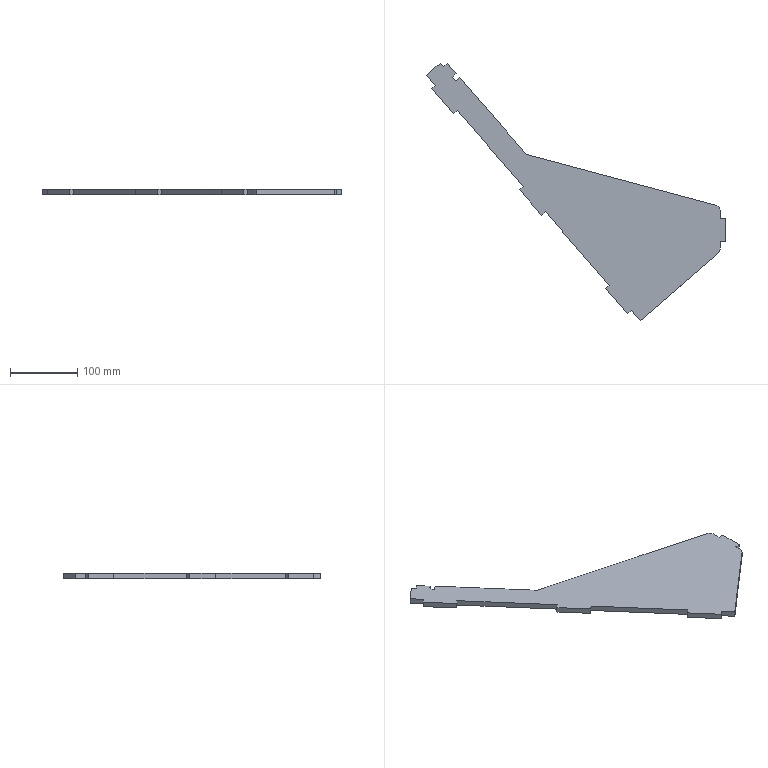Part | SolidWorks | features FlatPattern 1, SMBaseFlange 1, SheetMetal 1 | 1 solid | 33 faces | box 445.432 x 383.748 x 8 mm | volume 369427 mm3 | plane 30 | cylinder 3 | commonest cylinder face diameters 20 x2 4 x1
STEP:
#1=CARTESIAN_POINT('',(-13.039,-561.326,0.));
#2=VERTEX_POINT('',#1);
#3=CARTESIAN_POINT('',(-9.6,-553.779,0.));
#4=VERTEX_POINT('',#3);
#5=CARTESIAN_POINT('',(-19.6,-553.779,0.));
#6=DIRECTION('',(0.,0.,1.));
#7=DIRECTION('',(1.,0.,0.));
#8=AXIS2_PLACEMENT_3D('',#5,#6,#7);
#9=CIRCLE('',#8,10.);
#10=EDGE_CURVE('',#2,#4,#9,.T.);
#11=ORIENTED_EDGE('',*,*,#10,.F.);
#12=CARTESIAN_POINT('',(-13.039,-561.326,-8.));
#13=VERTEX_POINT('',#12);
#14=CARTESIAN_POINT('',(-13.039,-561.326,-8.));
#15=DIRECTION('',(0.,0.,1.));
#16=VECTOR('',#15,1000.);
#17=LINE('',#14,#16);
#18=EDGE_CURVE('',#13,#2,#17,.T.);
#19=ORIENTED_EDGE('',*,*,#18,.F.);
#20=CARTESIAN_POINT('',(-9.6,-553.779,-8.));
#21=VERTEX_POINT('',#20);
#22=CARTESIAN_POINT('',(-19.6,-553.779,-8.));
#23=DIRECTION('',(0.,0.,1.));
#24=DIRECTION('',(1.,0.,0.));
#25=AXIS2_PLACEMENT_3D('',#22,#23,#24);
#26=CIRCLE('',#25,10.);
#27=EDGE_CURVE('',#13,#21,#26,.T.);
#28=ORIENTED_EDGE('',*,*,#27,.T.);
#29=CARTESIAN_POINT('',(-9.6,-553.779,-8.));
#30=DIRECTION('',(0.,0.,1.));
#31=VECTOR('',#30,1000.);
#32=LINE('',#29,#31);
#33=EDGE_CURVE('',#21,#4,#32,.T.);
#34=ORIENTED_EDGE('',*,*,#33,.T.);
#35=EDGE_LOOP('',(#11,#19,#28,#34));
#36=FACE_OUTER_BOUND('',#35,.T.);
#37=CARTESIAN_POINT('',(-19.6,-553.779,-8.));
#38=DIRECTION('',(0.,0.,1.));
#39=DIRECTION('',(1.,0.,0.));
#40=AXIS2_PLACEMENT_3D('',#37,#38,#39);
#41=CYLINDRICAL_SURFACE('',#40,10.);
#42=ADVANCED_FACE('',(#36),#41,.T.);
#43=CARTESIAN_POINT('',(-129.344,-662.428,0.));
#44=VERTEX_POINT('',#43);
#45=CARTESIAN_POINT('',(-13.039,-561.326,0.));
#46=DIRECTION('',(0.7547,0.6561,0.));
#47=VECTOR('',#46,1000.);
#48=LINE('',#45,#47);
#49=EDGE_CURVE('',#44,#2,#48,.T.);
#50=ORIENTED_EDGE('',*,*,#49,.F.);
#51=CARTESIAN_POINT('',(-129.344,-662.428,-8.));
#52=VERTEX_POINT('',#51);
#53=CARTESIAN_POINT('',(-129.344,-662.428,-8.));
#54=DIRECTION('',(0.,0.,1.));
#55=VECTOR('',#54,1000.);
#56=LINE('',#53,#55);
#57=EDGE_CURVE('',#52,#44,#56,.T.);
#58=ORIENTED_EDGE('',*,*,#57,.F.);
#59=CARTESIAN_POINT('',(-13.039,-561.326,-8.));
#60=DIRECTION('',(0.7547,0.6561,0.));
#61=VECTOR('',#60,1000.);
#62=LINE('',#59,#61);
#63=EDGE_CURVE('',#52,#13,#62,.T.);
#64=ORIENTED_EDGE('',*,*,#63,.T.);
#65=ORIENTED_EDGE('',*,*,#18,.T.);
#66=EDGE_LOOP('',(#50,#58,#64,#65));
#67=FACE_OUTER_BOUND('',#66,.T.);
#68=CARTESIAN_POINT('',(-13.039,-561.326,-8.));
#69=DIRECTION('',(0.6561,-0.7547,0.));
#70=DIRECTION('',(0.7547,0.6561,0.));
#71=AXIS2_PLACEMENT_3D('',#68,#69,#70);
#72=PLANE('',#71);
#73=ADVANCED_FACE('',(#67),#72,.T.);
#74=CARTESIAN_POINT('',(-142.465,-647.333,0.));
#75=VERTEX_POINT('',#74);
#76=CARTESIAN_POINT('',(-142.465,-647.333,0.));
#77=DIRECTION('',(0.6561,-0.7547,0.));
#78=VECTOR('',#77,1000.);
#79=LINE('',#76,#78);
#80=EDGE_CURVE('',#75,#44,#79,.T.);
#81=ORIENTED_EDGE('',*,*,#80,.F.);
#82=CARTESIAN_POINT('',(-142.465,-647.333,-8.));
#83=VERTEX_POINT('',#82);
#84=CARTESIAN_POINT('',(-142.465,-647.333,-8.));
#85=DIRECTION('',(0.,0.,1.));
#86=VECTOR('',#85,1000.);
#87=LINE('',#84,#86);
#88=EDGE_CURVE('',#83,#75,#87,.T.);
#89=ORIENTED_EDGE('',*,*,#88,.F.);
#90=CARTESIAN_POINT('',(-142.465,-647.333,-8.));
#91=DIRECTION('',(0.6561,-0.7547,0.));
#92=VECTOR('',#91,1000.);
#93=LINE('',#90,#92);
#94=EDGE_CURVE('',#83,#52,#93,.T.);
#95=ORIENTED_EDGE('',*,*,#94,.T.);
#96=ORIENTED_EDGE('',*,*,#57,.T.);
#97=EDGE_LOOP('',(#81,#89,#95,#96));
#98=FACE_OUTER_BOUND('',#97,.T.);
#99=CARTESIAN_POINT('',(-142.465,-647.333,-8.));
#100=DIRECTION('',(-0.7547,-0.6561,0.));
#101=DIRECTION('',(0.6561,-0.7547,0.));
#102=AXIS2_PLACEMENT_3D('',#99,#100,#101);
#103=PLANE('',#102);
#104=ADVANCED_FACE('',(#98),#103,.T.);
#105=CARTESIAN_POINT('',(-148.125,-652.254,0.));
#106=VERTEX_POINT('',#105);
#107=CARTESIAN_POINT('',(-142.465,-647.333,0.));
#108=DIRECTION('',(0.7547,0.6561,0.));
#109=VECTOR('',#108,1000.);
#110=LINE('',#107,#109);
#111=EDGE_CURVE('',#106,#75,#110,.T.);
#112=ORIENTED_EDGE('',*,*,#111,.F.);
#113=CARTESIAN_POINT('',(-148.125,-652.254,-8.));
#114=VERTEX_POINT('',#113);
#115=CARTESIAN_POINT('',(-148.125,-652.254,-8.));
#116=DIRECTION('',(0.,0.,1.));
#117=VECTOR('',#116,1000.);
#118=LINE('',#115,#117);
#119=EDGE_CURVE('',#114,#106,#118,.T.);
#120=ORIENTED_EDGE('',*,*,#119,.F.);
#121=CARTESIAN_POINT('',(-142.465,-647.333,-8.));
#122=DIRECTION('',(0.7547,0.6561,0.));
#123=VECTOR('',#122,1000.);
#124=LINE('',#121,#123);
#125=EDGE_CURVE('',#114,#83,#124,.T.);
#126=ORIENTED_EDGE('',*,*,#125,.T.);
#127=ORIENTED_EDGE('',*,*,#88,.T.);
#128=EDGE_LOOP('',(#112,#120,#126,#127));
#129=FACE_OUTER_BOUND('',#128,.T.);
#130=CARTESIAN_POINT('',(-142.465,-647.333,-8.));
#131=DIRECTION('',(0.6561,-0.7547,0.));
#132=DIRECTION('',(0.7547,0.6561,0.));
#133=AXIS2_PLACEMENT_3D('',#130,#131,#132);
#134=PLANE('',#133);
#135=ADVANCED_FACE('',(#129),#134,.T.);
#136=CARTESIAN_POINT('',(-180.928,-614.518,0.));
#137=VERTEX_POINT('',#136);
#138=CARTESIAN_POINT('',(-148.125,-652.254,0.));
#139=DIRECTION('',(0.6561,-0.7547,0.));
#140=VECTOR('',#139,1000.);
#141=LINE('',#138,#140);
#142=EDGE_CURVE('',#137,#106,#141,.T.);
#143=ORIENTED_EDGE('',*,*,#142,.F.);
#144=CARTESIAN_POINT('',(-180.928,-614.518,-8.));
#145=VERTEX_POINT('',#144);
#146=CARTESIAN_POINT('',(-180.928,-614.518,-8.));
#147=DIRECTION('',(0.,0.,1.));
#148=VECTOR('',#147,1000.);
#149=LINE('',#146,#148);
#150=EDGE_CURVE('',#145,#137,#149,.T.);
#151=ORIENTED_EDGE('',*,*,#150,.F.);
#152=CARTESIAN_POINT('',(-148.125,-652.254,-8.));
#153=DIRECTION('',(0.6561,-0.7547,0.));
#154=VECTOR('',#153,1000.);
#155=LINE('',#152,#154);
#156=EDGE_CURVE('',#145,#114,#155,.T.);
#157=ORIENTED_EDGE('',*,*,#156,.T.);
#158=ORIENTED_EDGE('',*,*,#119,.T.);
#159=EDGE_LOOP('',(#143,#151,#157,#158));
#160=FACE_OUTER_BOUND('',#159,.T.);
#161=CARTESIAN_POINT('',(-148.125,-652.254,-8.));
#162=DIRECTION('',(-0.7547,-0.6561,0.));
#163=DIRECTION('',(0.6561,-0.7547,0.));
#164=AXIS2_PLACEMENT_3D('',#161,#162,#163);
#165=PLANE('',#164);
#166=ADVANCED_FACE('',(#160),#165,.T.);
#167=CARTESIAN_POINT('',(-175.268,-609.598,0.));
#168=VERTEX_POINT('',#167);
#169=CARTESIAN_POINT('',(-180.928,-614.518,0.));
#170=DIRECTION('',(-0.7547,-0.6561,0.));
#171=VECTOR('',#170,1000.);
#172=LINE('',#169,#171);
#173=EDGE_CURVE('',#168,#137,#172,.T.);
#174=ORIENTED_EDGE('',*,*,#173,.F.);
#175=CARTESIAN_POINT('',(-175.268,-609.598,-8.));
#176=VERTEX_POINT('',#175);
#177=CARTESIAN_POINT('',(-175.268,-609.598,-8.));
#178=DIRECTION('',(0.,0.,1.));
#179=VECTOR('',#178,1000.);
#180=LINE('',#177,#179);
#181=EDGE_CURVE('',#176,#168,#180,.T.);
#182=ORIENTED_EDGE('',*,*,#181,.F.);
#183=CARTESIAN_POINT('',(-180.928,-614.518,-8.));
#184=DIRECTION('',(-0.7547,-0.6561,0.));
#185=VECTOR('',#184,1000.);
#186=LINE('',#183,#185);
#187=EDGE_CURVE('',#176,#145,#186,.T.);
#188=ORIENTED_EDGE('',*,*,#187,.T.);
#189=ORIENTED_EDGE('',*,*,#150,.T.);
#190=EDGE_LOOP('',(#174,#182,#188,#189));
#191=FACE_OUTER_BOUND('',#190,.T.);
#192=CARTESIAN_POINT('',(-180.928,-614.518,-8.));
#193=DIRECTION('',(-0.6561,0.7547,0.));
#194=DIRECTION('',(-0.7547,-0.6561,0.));
#195=AXIS2_PLACEMENT_3D('',#192,#193,#194);
#196=PLANE('',#195);
#197=ADVANCED_FACE('',(#191),#196,.T.);
#198=CARTESIAN_POINT('',(-270.396,-500.165,0.));
#199=VERTEX_POINT('',#198);
#200=CARTESIAN_POINT('',(-270.396,-500.165,0.));
#201=DIRECTION('',(0.6561,-0.7547,0.));
#202=VECTOR('',#201,1000.);
#203=LINE('',#200,#202);
#204=EDGE_CURVE('',#199,#168,#203,.T.);
#205=ORIENTED_EDGE('',*,*,#204,.F.);
#206=CARTESIAN_POINT('',(-270.396,-500.165,-8.));
#207=VERTEX_POINT('',#206);
#208=CARTESIAN_POINT('',(-270.396,-500.165,-8.));
#209=DIRECTION('',(0.,0.,1.));
#210=VECTOR('',#209,1000.);
#211=LINE('',#208,#210);
#212=EDGE_CURVE('',#207,#199,#211,.T.);
#213=ORIENTED_EDGE('',*,*,#212,.F.);
#214=CARTESIAN_POINT('',(-270.396,-500.165,-8.));
#215=DIRECTION('',(0.6561,-0.7547,0.));
#216=VECTOR('',#215,1000.);
#217=LINE('',#214,#216);
#218=EDGE_CURVE('',#207,#176,#217,.T.);
#219=ORIENTED_EDGE('',*,*,#218,.T.);
#220=ORIENTED_EDGE('',*,*,#181,.T.);
#221=EDGE_LOOP('',(#205,#213,#219,#220));
#222=FACE_OUTER_BOUND('',#221,.T.);
#223=CARTESIAN_POINT('',(-270.396,-500.165,-8.));
#224=DIRECTION('',(-0.7547,-0.6561,0.));
#225=DIRECTION('',(0.6561,-0.7547,0.));
#226=AXIS2_PLACEMENT_3D('',#223,#224,#225);
#227=PLANE('',#226);
#228=ADVANCED_FACE('',(#222),#227,.T.);
#229=CARTESIAN_POINT('',(-276.057,-505.085,0.));
#230=VERTEX_POINT('',#229);
#231=CARTESIAN_POINT('',(-276.057,-505.085,0.));
#232=DIRECTION('',(0.7547,0.6561,0.));
#233=VECTOR('',#232,1000.);
#234=LINE('',#231,#233);
#235=EDGE_CURVE('',#230,#199,#234,.T.);
#236=ORIENTED_EDGE('',*,*,#235,.F.);
#237=CARTESIAN_POINT('',(-276.057,-505.085,-8.));
#238=VERTEX_POINT('',#237);
#239=CARTESIAN_POINT('',(-276.057,-505.085,-8.));
#240=DIRECTION('',(0.,0.,1.));
#241=VECTOR('',#240,1000.);
#242=LINE('',#239,#241);
#243=EDGE_CURVE('',#238,#230,#242,.T.);
#244=ORIENTED_EDGE('',*,*,#243,.F.);
#245=CARTESIAN_POINT('',(-276.057,-505.085,-8.));
#246=DIRECTION('',(0.7547,0.6561,0.));
#247=VECTOR('',#246,1000.);
#248=LINE('',#245,#247);
#249=EDGE_CURVE('',#238,#207,#248,.T.);
#250=ORIENTED_EDGE('',*,*,#249,.T.);
#251=ORIENTED_EDGE('',*,*,#212,.T.);
#252=EDGE_LOOP('',(#236,#244,#250,#251));
#253=FACE_OUTER_BOUND('',#252,.T.);
#254=CARTESIAN_POINT('',(-276.057,-505.085,-8.));
#255=DIRECTION('',(0.6561,-0.7547,0.));
#256=DIRECTION('',(0.7547,0.6561,0.));
#257=AXIS2_PLACEMENT_3D('',#254,#255,#256);
#258=PLANE('',#257);
#259=ADVANCED_FACE('',(#253),#258,.T.);
#260=CARTESIAN_POINT('',(-308.86,-467.35,0.));
#261=VERTEX_POINT('',#260);
#262=CARTESIAN_POINT('',(-308.86,-467.35,0.));
#263=DIRECTION('',(0.6561,-0.7547,0.));
#264=VECTOR('',#263,1000.);
#265=LINE('',#262,#264);
#266=EDGE_CURVE('',#261,#230,#265,.T.);
#267=ORIENTED_EDGE('',*,*,#266,.F.);
#268=CARTESIAN_POINT('',(-308.86,-467.35,-8.));
#269=VERTEX_POINT('',#268);
#270=CARTESIAN_POINT('',(-308.86,-467.35,-8.));
#271=DIRECTION('',(0.,0.,1.));
#272=VECTOR('',#271,1000.);
#273=LINE('',#270,#272);
#274=EDGE_CURVE('',#269,#261,#273,.T.);
#275=ORIENTED_EDGE('',*,*,#274,.F.);
#276=CARTESIAN_POINT('',(-308.86,-467.35,-8.));
#277=DIRECTION('',(0.6561,-0.7547,0.));
#278=VECTOR('',#277,1000.);
#279=LINE('',#276,#278);
#280=EDGE_CURVE('',#269,#238,#279,.T.);
#281=ORIENTED_EDGE('',*,*,#280,.T.);
#282=ORIENTED_EDGE('',*,*,#243,.T.);
#283=EDGE_LOOP('',(#267,#275,#281,#282));
#284=FACE_OUTER_BOUND('',#283,.T.);
#285=CARTESIAN_POINT('',(-308.86,-467.35,-8.));
#286=DIRECTION('',(-0.7547,-0.6561,0.));
#287=DIRECTION('',(0.6561,-0.7547,0.));
#288=AXIS2_PLACEMENT_3D('',#285,#286,#287);
#289=PLANE('',#288);
#290=ADVANCED_FACE('',(#284),#289,.T.);
#291=CARTESIAN_POINT('',(-303.199,-462.429,0.));
#292=VERTEX_POINT('',#291);
#293=CARTESIAN_POINT('',(-303.199,-462.429,0.));
#294=DIRECTION('',(-0.7547,-0.6561,0.));
#295=VECTOR('',#294,1000.);
#296=LINE('',#293,#295);
#297=EDGE_CURVE('',#292,#261,#296,.T.);
#298=ORIENTED_EDGE('',*,*,#297,.F.);
#299=CARTESIAN_POINT('',(-303.199,-462.429,-8.));
#300=VERTEX_POINT('',#299);
#301=CARTESIAN_POINT('',(-303.199,-462.429,-8.));
#302=DIRECTION('',(0.,0.,1.));
#303=VECTOR('',#302,1000.);
#304=LINE('',#301,#303);
#305=EDGE_CURVE('',#300,#292,#304,.T.);
#306=ORIENTED_EDGE('',*,*,#305,.F.);
#307=CARTESIAN_POINT('',(-303.199,-462.429,-8.));
#308=DIRECTION('',(-0.7547,-0.6561,0.));
#309=VECTOR('',#308,1000.);
#310=LINE('',#307,#309);
#311=EDGE_CURVE('',#300,#269,#310,.T.);
#312=ORIENTED_EDGE('',*,*,#311,.T.);
#313=ORIENTED_EDGE('',*,*,#274,.T.);
#314=EDGE_LOOP('',(#298,#306,#312,#313));
#315=FACE_OUTER_BOUND('',#314,.T.);
#316=CARTESIAN_POINT('',(-303.199,-462.429,-8.));
#317=DIRECTION('',(-0.6561,0.7547,0.));
#318=DIRECTION('',(-0.7547,-0.6561,0.));
#319=AXIS2_PLACEMENT_3D('',#316,#317,#318);
#320=PLANE('',#319);
#321=ADVANCED_FACE('',(#315),#320,.T.);
#322=CARTESIAN_POINT('',(-401.608,-349.223,0.));
#323=VERTEX_POINT('',#322);
#324=CARTESIAN_POINT('',(-401.608,-349.223,0.));
#325=DIRECTION('',(0.6561,-0.7547,0.));
#326=VECTOR('',#325,1000.);
#327=LINE('',#324,#326);
#328=EDGE_CURVE('',#323,#292,#327,.T.);
#329=ORIENTED_EDGE('',*,*,#328,.F.);
#330=CARTESIAN_POINT('',(-401.608,-349.223,-8.));
#331=VERTEX_POINT('',#330);
#332=CARTESIAN_POINT('',(-401.608,-349.223,-8.));
#333=DIRECTION('',(0.,0.,1.));
#334=VECTOR('',#333,1000.);
#335=LINE('',#332,#334);
#336=EDGE_CURVE('',#331,#323,#335,.T.);
#337=ORIENTED_EDGE('',*,*,#336,.F.);
#338=CARTESIAN_POINT('',(-401.608,-349.223,-8.));
#339=DIRECTION('',(0.6561,-0.7547,0.));
#340=VECTOR('',#339,1000.);
#341=LINE('',#338,#340);
#342=EDGE_CURVE('',#331,#300,#341,.T.);
#343=ORIENTED_EDGE('',*,*,#342,.T.);
#344=ORIENTED_EDGE('',*,*,#305,.T.);
#345=EDGE_LOOP('',(#329,#337,#343,#344));
#346=FACE_OUTER_BOUND('',#345,.T.);
#347=CARTESIAN_POINT('',(-401.608,-349.223,-8.));
#348=DIRECTION('',(-0.7547,-0.6561,0.));
#349=DIRECTION('',(0.6561,-0.7547,0.));
#350=AXIS2_PLACEMENT_3D('',#347,#348,#349);
#351=PLANE('',#350);
#352=ADVANCED_FACE('',(#346),#351,.T.);
#353=CARTESIAN_POINT('',(-407.269,-354.143,0.));
#354=VERTEX_POINT('',#353);
#355=CARTESIAN_POINT('',(-407.269,-354.143,0.));
#356=DIRECTION('',(0.7547,0.6561,0.));
#357=VECTOR('',#356,1000.);
#358=LINE('',#355,#357);
#359=EDGE_CURVE('',#354,#323,#358,.T.);
#360=ORIENTED_EDGE('',*,*,#359,.F.);
#361=CARTESIAN_POINT('',(-407.269,-354.143,-8.));
#362=VERTEX_POINT('',#361);
#363=CARTESIAN_POINT('',(-407.269,-354.143,-8.));
#364=DIRECTION('',(0.,0.,1.));
#365=VECTOR('',#364,1000.);
#366=LINE('',#363,#365);
#367=EDGE_CURVE('',#362,#354,#366,.T.);
#368=ORIENTED_EDGE('',*,*,#367,.F.);
#369=CARTESIAN_POINT('',(-407.269,-354.143,-8.));
#370=DIRECTION('',(0.7547,0.6561,0.));
#371=VECTOR('',#370,1000.);
#372=LINE('',#369,#371);
#373=EDGE_CURVE('',#362,#331,#372,.T.);
#374=ORIENTED_EDGE('',*,*,#373,.T.);
#375=ORIENTED_EDGE('',*,*,#336,.T.);
#376=EDGE_LOOP('',(#360,#368,#374,#375));
#377=FACE_OUTER_BOUND('',#376,.T.);
#378=CARTESIAN_POINT('',(-407.269,-354.143,-8.));
#379=DIRECTION('',(0.6561,-0.7547,0.));
#380=DIRECTION('',(0.7547,0.6561,0.));
#381=AXIS2_PLACEMENT_3D('',#378,#379,#380);
#382=PLANE('',#381);
#383=ADVANCED_FACE('',(#377),#382,.T.);
#384=CARTESIAN_POINT('',(-440.071,-316.408,0.));
#385=VERTEX_POINT('',#384);
#386=CARTESIAN_POINT('',(-440.071,-316.408,0.));
#387=DIRECTION('',(0.6561,-0.7547,0.));
#388=VECTOR('',#387,1000.);
#389=LINE('',#386,#388);
#390=EDGE_CURVE('',#385,#354,#389,.T.);
#391=ORIENTED_EDGE('',*,*,#390,.F.);
#392=CARTESIAN_POINT('',(-440.071,-316.408,-8.));
#393=VERTEX_POINT('',#392);
#394=CARTESIAN_POINT('',(-440.071,-316.408,-8.));
#395=DIRECTION('',(0.,0.,1.));
#396=VECTOR('',#395,1000.);
#397=LINE('',#394,#396);
#398=EDGE_CURVE('',#393,#385,#397,.T.);
#399=ORIENTED_EDGE('',*,*,#398,.F.);
#400=CARTESIAN_POINT('',(-440.071,-316.408,-8.));
#401=DIRECTION('',(0.6561,-0.7547,0.));
#402=VECTOR('',#401,1000.);
#403=LINE('',#400,#402);
#404=EDGE_CURVE('',#393,#362,#403,.T.);
#405=ORIENTED_EDGE('',*,*,#404,.T.);
#406=ORIENTED_EDGE('',*,*,#367,.T.);
#407=EDGE_LOOP('',(#391,#399,#405,#406));
#408=FACE_OUTER_BOUND('',#407,.T.);
#409=CARTESIAN_POINT('',(-440.071,-316.408,-8.));
#410=DIRECTION('',(-0.7547,-0.6561,0.));
#411=DIRECTION('',(0.6561,-0.7547,0.));
#412=AXIS2_PLACEMENT_3D('',#409,#410,#411);
#413=PLANE('',#412);
#414=ADVANCED_FACE('',(#408),#413,.T.);
#415=CARTESIAN_POINT('',(-434.411,-311.488,0.));
#416=VERTEX_POINT('',#415);
#417=CARTESIAN_POINT('',(-434.411,-311.488,0.));
#418=DIRECTION('',(-0.7547,-0.6561,0.));
#419=VECTOR('',#418,1000.);
#420=LINE('',#417,#419);
#421=EDGE_CURVE('',#416,#385,#420,.T.);
#422=ORIENTED_EDGE('',*,*,#421,.F.);
#423=CARTESIAN_POINT('',(-434.411,-311.488,-8.));
#424=VERTEX_POINT('',#423);
#425=CARTESIAN_POINT('',(-434.411,-311.488,-8.));
#426=DIRECTION('',(0.,0.,1.));
#427=VECTOR('',#426,1000.);
#428=LINE('',#425,#427);
#429=EDGE_CURVE('',#424,#416,#428,.T.);
#430=ORIENTED_EDGE('',*,*,#429,.F.);
#431=CARTESIAN_POINT('',(-434.411,-311.488,-8.));
#432=DIRECTION('',(-0.7547,-0.6561,0.));
#433=VECTOR('',#432,1000.);
#434=LINE('',#431,#433);
#435=EDGE_CURVE('',#424,#393,#434,.T.);
#436=ORIENTED_EDGE('',*,*,#435,.T.);
#437=ORIENTED_EDGE('',*,*,#398,.T.);
#438=EDGE_LOOP('',(#422,#430,#436,#437));
#439=FACE_OUTER_BOUND('',#438,.T.);
#440=CARTESIAN_POINT('',(-434.411,-311.488,-8.));
#441=DIRECTION('',(-0.6561,0.7547,0.));
#442=DIRECTION('',(-0.7547,-0.6561,0.));
#443=AXIS2_PLACEMENT_3D('',#440,#441,#442);
#444=PLANE('',#443);
#445=ADVANCED_FACE('',(#439),#444,.T.);
#446=CARTESIAN_POINT('',(-447.532,-296.393,0.));
#447=VERTEX_POINT('',#446);
#448=CARTESIAN_POINT('',(-447.532,-296.393,0.));
#449=DIRECTION('',(0.6561,-0.7547,0.));
#450=VECTOR('',#449,1000.);
#451=LINE('',#448,#450);
#452=EDGE_CURVE('',#447,#416,#451,.T.);
#453=ORIENTED_EDGE('',*,*,#452,.F.);
#454=CARTESIAN_POINT('',(-447.532,-296.393,-8.));
#455=VERTEX_POINT('',#454);
#456=CARTESIAN_POINT('',(-447.532,-296.393,-8.));
#457=DIRECTION('',(0.,0.,1.));
#458=VECTOR('',#457,1000.);
#459=LINE('',#456,#458);
#460=EDGE_CURVE('',#455,#447,#459,.T.);
#461=ORIENTED_EDGE('',*,*,#460,.F.);
#462=CARTESIAN_POINT('',(-447.532,-296.393,-8.));
#463=DIRECTION('',(0.6561,-0.7547,0.));
#464=VECTOR('',#463,1000.);
#465=LINE('',#462,#464);
#466=EDGE_CURVE('',#455,#424,#465,.T.);
#467=ORIENTED_EDGE('',*,*,#466,.T.);
#468=ORIENTED_EDGE('',*,*,#429,.T.);
#469=EDGE_LOOP('',(#453,#461,#467,#468));
#470=FACE_OUTER_BOUND('',#469,.T.);
#471=CARTESIAN_POINT('',(-447.532,-296.393,-8.));
#472=DIRECTION('',(-0.7547,-0.6561,0.));
#473=DIRECTION('',(0.6561,-0.7547,0.));
#474=AXIS2_PLACEMENT_3D('',#471,#472,#473);
#475=PLANE('',#474);
#476=ADVANCED_FACE('',(#470),#475,.T.);
#477=CARTESIAN_POINT('',(-427.155,-278.68,0.));
#478=VERTEX_POINT('',#477);
#479=CARTESIAN_POINT('',(-427.155,-278.68,0.));
#480=DIRECTION('',(-0.7547,-0.6561,0.));
#481=VECTOR('',#480,1000.);
#482=LINE('',#479,#481);
#483=EDGE_CURVE('',#478,#447,#482,.T.);
#484=ORIENTED_EDGE('',*,*,#483,.F.);
#485=CARTESIAN_POINT('',(-427.155,-278.68,-8.));
#486=VERTEX_POINT('',#485);
#487=CARTESIAN_POINT('',(-427.155,-278.68,-8.));
#488=DIRECTION('',(0.,0.,1.));
#489=VECTOR('',#488,1000.);
#490=LINE('',#487,#489);
#491=EDGE_CURVE('',#486,#478,#490,.T.);
#492=ORIENTED_EDGE('',*,*,#491,.F.);
#493=CARTESIAN_POINT('',(-427.155,-278.68,-8.));
#494=DIRECTION('',(-0.7547,-0.6561,0.));
#495=VECTOR('',#494,1000.);
#496=LINE('',#493,#495);
#497=EDGE_CURVE('',#486,#455,#496,.T.);
#498=ORIENTED_EDGE('',*,*,#497,.T.);
#499=ORIENTED_EDGE('',*,*,#460,.T.);
#500=EDGE_LOOP('',(#484,#492,#498,#499));
#501=FACE_OUTER_BOUND('',#500,.T.);
#502=CARTESIAN_POINT('',(-427.155,-278.68,-8.));
#503=DIRECTION('',(-0.6561,0.7547,0.));
#504=DIRECTION('',(-0.7547,-0.6561,0.));
#505=AXIS2_PLACEMENT_3D('',#502,#503,#504);
#506=PLANE('',#505);
#507=ADVANCED_FACE('',(#501),#506,.T.);
#508=CARTESIAN_POINT('',(-422.235,-284.34,0.));
#509=VERTEX_POINT('',#508);
#510=CARTESIAN_POINT('',(-427.155,-278.68,0.));
#511=DIRECTION('',(-0.6561,0.7547,0.));
#512=VECTOR('',#511,1000.);
#513=LINE('',#510,#512);
#514=EDGE_CURVE('',#509,#478,#513,.T.);
#515=ORIENTED_EDGE('',*,*,#514,.F.);
#516=CARTESIAN_POINT('',(-422.235,-284.34,-8.));
#517=VERTEX_POINT('',#516);
#518=CARTESIAN_POINT('',(-422.235,-284.34,-8.));
#519=DIRECTION('',(0.,0.,1.));
#520=VECTOR('',#519,1000.);
#521=LINE('',#518,#520);
#522=EDGE_CURVE('',#517,#509,#521,.T.);
#523=ORIENTED_EDGE('',*,*,#522,.F.);
#524=CARTESIAN_POINT('',(-427.155,-278.68,-8.));
#525=DIRECTION('',(-0.6561,0.7547,0.));
#526=VECTOR('',#525,1000.);
#527=LINE('',#524,#526);
#528=EDGE_CURVE('',#517,#486,#527,.T.);
#529=ORIENTED_EDGE('',*,*,#528,.T.);
#530=ORIENTED_EDGE('',*,*,#491,.T.);
#531=EDGE_LOOP('',(#515,#523,#529,#530));
#532=FACE_OUTER_BOUND('',#531,.T.);
#533=CARTESIAN_POINT('',(-427.155,-278.68,-8.));
#534=DIRECTION('',(0.7547,0.6561,0.));
#535=DIRECTION('',(-0.6561,0.7547,0.));
#536=AXIS2_PLACEMENT_3D('',#533,#534,#535);
#537=PLANE('',#536);
#538=ADVANCED_FACE('',(#532),#537,.T.);
#539=CARTESIAN_POINT('',(-416.574,-279.42,0.));
#540=VERTEX_POINT('',#539);
#541=CARTESIAN_POINT('',(-422.235,-284.34,0.));
#542=DIRECTION('',(-0.7547,-0.6561,0.));
#543=VECTOR('',#542,1000.);
#544=LINE('',#541,#543);
#545=EDGE_CURVE('',#540,#509,#544,.T.);
#546=ORIENTED_EDGE('',*,*,#545,.F.);
#547=CARTESIAN_POINT('',(-416.574,-279.42,-8.));
#548=VERTEX_POINT('',#547);
#549=CARTESIAN_POINT('',(-416.574,-279.42,-8.));
#550=DIRECTION('',(0.,0.,1.));
#551=VECTOR('',#550,1000.);
#552=LINE('',#549,#551);
#553=EDGE_CURVE('',#548,#540,#552,.T.);
#554=ORIENTED_EDGE('',*,*,#553,.F.);
#555=CARTESIAN_POINT('',(-422.235,-284.34,-8.));
#556=DIRECTION('',(-0.7547,-0.6561,0.));
#557=VECTOR('',#556,1000.);
#558=LINE('',#555,#557);
#559=EDGE_CURVE('',#548,#517,#558,.T.);
#560=ORIENTED_EDGE('',*,*,#559,.T.);
#561=ORIENTED_EDGE('',*,*,#522,.T.);
#562=EDGE_LOOP('',(#546,#554,#560,#561));
#563=FACE_OUTER_BOUND('',#562,.T.);
#564=CARTESIAN_POINT('',(-422.235,-284.34,-8.));
#565=DIRECTION('',(-0.6561,0.7547,0.));
#566=DIRECTION('',(-0.7547,-0.6561,0.));
#567=AXIS2_PLACEMENT_3D('',#564,#565,#566);
#568=PLANE('',#567);
#569=ADVANCED_FACE('',(#563),#568,.T.);
#570=CARTESIAN_POINT('',(-403.453,-294.514,0.));
#571=VERTEX_POINT('',#570);
#572=CARTESIAN_POINT('',(-416.574,-279.42,0.));
#573=DIRECTION('',(-0.6561,0.7547,0.));
#574=VECTOR('',#573,1000.);
#575=LINE('',#572,#574);
#576=EDGE_CURVE('',#571,#540,#575,.T.);
#577=ORIENTED_EDGE('',*,*,#576,.F.);
#578=CARTESIAN_POINT('',(-403.453,-294.514,-8.));
#579=VERTEX_POINT('',#578);
#580=CARTESIAN_POINT('',(-403.453,-294.514,-8.));
#581=DIRECTION('',(0.,0.,1.));
#582=VECTOR('',#581,1000.);
#583=LINE('',#580,#582);
#584=EDGE_CURVE('',#579,#571,#583,.T.);
#585=ORIENTED_EDGE('',*,*,#584,.F.);
#586=CARTESIAN_POINT('',(-416.574,-279.42,-8.));
#587=DIRECTION('',(-0.6561,0.7547,0.));
#588=VECTOR('',#587,1000.);
#589=LINE('',#586,#588);
#590=EDGE_CURVE('',#579,#548,#589,.T.);
#591=ORIENTED_EDGE('',*,*,#590,.T.);
#592=ORIENTED_EDGE('',*,*,#553,.T.);
#593=EDGE_LOOP('',(#577,#585,#591,#592));
#594=FACE_OUTER_BOUND('',#593,.T.);
#595=CARTESIAN_POINT('',(-416.574,-279.42,-8.));
#596=DIRECTION('',(0.7547,0.6561,0.));
#597=DIRECTION('',(-0.6561,0.7547,0.));
#598=AXIS2_PLACEMENT_3D('',#595,#596,#597);
#599=PLANE('',#598);
#600=ADVANCED_FACE('',(#594),#599,.T.);
#601=CARTESIAN_POINT('',(-409.114,-299.434,0.));
#602=VERTEX_POINT('',#601);
#603=CARTESIAN_POINT('',(-403.453,-294.514,0.));
#604=DIRECTION('',(0.7547,0.6561,0.));
#605=VECTOR('',#604,1000.);
#606=LINE('',#603,#605);
#607=EDGE_CURVE('',#602,#571,#606,.T.);
#608=ORIENTED_EDGE('',*,*,#607,.F.);
#609=CARTESIAN_POINT('',(-409.114,-299.434,-8.));
#610=VERTEX_POINT('',#609);
#611=CARTESIAN_POINT('',(-409.114,-299.434,-8.));
#612=DIRECTION('',(0.,0.,1.));
#613=VECTOR('',#612,1000.);
#614=LINE('',#611,#613);
#615=EDGE_CURVE('',#610,#602,#614,.T.);
#616=ORIENTED_EDGE('',*,*,#615,.F.);
#617=CARTESIAN_POINT('',(-403.453,-294.514,-8.));
#618=DIRECTION('',(0.7547,0.6561,0.));
#619=VECTOR('',#618,1000.);
#620=LINE('',#617,#619);
#621=EDGE_CURVE('',#610,#579,#620,.T.);
#622=ORIENTED_EDGE('',*,*,#621,.T.);
#623=ORIENTED_EDGE('',*,*,#584,.T.);
#624=EDGE_LOOP('',(#608,#616,#622,#623));
#625=FACE_OUTER_BOUND('',#624,.T.);
#626=CARTESIAN_POINT('',(-403.453,-294.514,-8.));
#627=DIRECTION('',(0.6561,-0.7547,0.));
#628=DIRECTION('',(0.7547,0.6561,0.));
#629=AXIS2_PLACEMENT_3D('',#626,#627,#628);
#630=PLANE('',#629);
#631=ADVANCED_FACE('',(#625),#630,.T.);
#632=CARTESIAN_POINT('',(-404.193,-305.095,0.));
#633=VERTEX_POINT('',#632);
#634=CARTESIAN_POINT('',(-409.114,-299.434,0.));
#635=DIRECTION('',(-0.6561,0.7547,0.));
#636=VECTOR('',#635,1000.);
#637=LINE('',#634,#636);
#638=EDGE_CURVE('',#633,#602,#637,.T.);
#639=ORIENTED_EDGE('',*,*,#638,.F.);
#640=CARTESIAN_POINT('',(-404.193,-305.095,-8.));
#641=VERTEX_POINT('',#640);
#642=CARTESIAN_POINT('',(-404.193,-305.095,-8.));
#643=DIRECTION('',(0.,0.,1.));
#644=VECTOR('',#643,1000.);
#645=LINE('',#642,#644);
#646=EDGE_CURVE('',#641,#633,#645,.T.);
#647=ORIENTED_EDGE('',*,*,#646,.F.);
#648=CARTESIAN_POINT('',(-409.114,-299.434,-8.));
#649=DIRECTION('',(-0.6561,0.7547,0.));
#650=VECTOR('',#649,1000.);
#651=LINE('',#648,#650);
#652=EDGE_CURVE('',#641,#610,#651,.T.);
#653=ORIENTED_EDGE('',*,*,#652,.T.);
#654=ORIENTED_EDGE('',*,*,#615,.T.);
#655=EDGE_LOOP('',(#639,#647,#653,#654));
#656=FACE_OUTER_BOUND('',#655,.T.);
#657=CARTESIAN_POINT('',(-409.114,-299.434,-8.));
#658=DIRECTION('',(0.7547,0.6561,0.));
#659=DIRECTION('',(-0.6561,0.7547,0.));
#660=AXIS2_PLACEMENT_3D('',#657,#658,#659);
#661=PLANE('',#660);
#662=ADVANCED_FACE('',(#656),#661,.T.);
#663=CARTESIAN_POINT('',(-398.155,-299.846,0.));
#664=VERTEX_POINT('',#663);
#665=CARTESIAN_POINT('',(-404.193,-305.095,0.));
#666=DIRECTION('',(-0.7547,-0.6561,0.));
#667=VECTOR('',#666,1000.);
#668=LINE('',#665,#667);
#669=EDGE_CURVE('',#664,#633,#668,.T.);
#670=ORIENTED_EDGE('',*,*,#669,.F.);
#671=CARTESIAN_POINT('',(-398.155,-299.846,-8.));
#672=VERTEX_POINT('',#671);
#673=CARTESIAN_POINT('',(-398.155,-299.846,-8.));
#674=DIRECTION('',(0.,0.,1.));
#675=VECTOR('',#674,1000.);
#676=LINE('',#673,#675);
#677=EDGE_CURVE('',#672,#664,#676,.T.);
#678=ORIENTED_EDGE('',*,*,#677,.F.);
#679=CARTESIAN_POINT('',(-404.193,-305.095,-8.));
#680=DIRECTION('',(-0.7547,-0.6561,0.));
#681=VECTOR('',#680,1000.);
#682=LINE('',#679,#681);
#683=EDGE_CURVE('',#672,#641,#682,.T.);
#684=ORIENTED_EDGE('',*,*,#683,.T.);
#685=ORIENTED_EDGE('',*,*,#646,.T.);
#686=EDGE_LOOP('',(#670,#678,#684,#685));
#687=FACE_OUTER_BOUND('',#686,.T.);
#688=CARTESIAN_POINT('',(-404.193,-305.095,-8.));
#689=DIRECTION('',(-0.6561,0.7547,0.));
#690=DIRECTION('',(-0.7547,-0.6561,0.));
#691=AXIS2_PLACEMENT_3D('',#688,#689,#690);
#692=PLANE('',#691);
#693=ADVANCED_FACE('',(#687),#692,.T.);
#694=CARTESIAN_POINT('',(-298.63,-414.337,0.));
#695=VERTEX_POINT('',#694);
#696=CARTESIAN_POINT('',(-398.155,-299.846,0.));
#697=DIRECTION('',(-0.6561,0.7547,0.));
#698=VECTOR('',#697,1000.);
#699=LINE('',#696,#698);
#700=EDGE_CURVE('',#695,#664,#699,.T.);
#701=ORIENTED_EDGE('',*,*,#700,.F.);
#702=CARTESIAN_POINT('',(-298.63,-414.337,-8.));
#703=VERTEX_POINT('',#702);
#704=CARTESIAN_POINT('',(-298.63,-414.337,-8.));
#705=DIRECTION('',(0.,0.,1.));
#706=VECTOR('',#705,1000.);
#707=LINE('',#704,#706);
#708=EDGE_CURVE('',#703,#695,#707,.T.);
#709=ORIENTED_EDGE('',*,*,#708,.F.);
#710=CARTESIAN_POINT('',(-398.155,-299.846,-8.));
#711=DIRECTION('',(-0.6561,0.7547,0.));
#712=VECTOR('',#711,1000.);
#713=LINE('',#710,#712);
#714=EDGE_CURVE('',#703,#672,#713,.T.);
#715=ORIENTED_EDGE('',*,*,#714,.T.);
#716=ORIENTED_EDGE('',*,*,#677,.T.);
#717=EDGE_LOOP('',(#701,#709,#715,#716));
#718=FACE_OUTER_BOUND('',#717,.T.);
#719=CARTESIAN_POINT('',(-398.155,-299.846,-8.));
#720=DIRECTION('',(0.7547,0.6561,0.));
#721=DIRECTION('',(-0.6561,0.7547,0.));
#722=AXIS2_PLACEMENT_3D('',#719,#720,#721);
#723=PLANE('',#722);
#724=ADVANCED_FACE('',(#718),#723,.T.);
#725=CARTESIAN_POINT('',(-297.639,-414.956,0.));
#726=VERTEX_POINT('',#725);
#727=CARTESIAN_POINT('',(-297.121,-413.024,0.));
#728=DIRECTION('',(0.,0.,-1.));
#729=DIRECTION('',(-1.,0.,0.));
#730=AXIS2_PLACEMENT_3D('',#727,#728,#729);
#731=CIRCLE('',#730,2.);
#732=EDGE_CURVE('',#726,#695,#731,.T.);
#733=ORIENTED_EDGE('',*,*,#732,.F.);
#734=CARTESIAN_POINT('',(-297.639,-414.956,-8.));
#735=VERTEX_POINT('',#734);
#736=CARTESIAN_POINT('',(-297.639,-414.956,-8.));
#737=DIRECTION('',(0.,0.,1.));
#738=VECTOR('',#737,1000.);
#739=LINE('',#736,#738);
#740=EDGE_CURVE('',#735,#726,#739,.T.);
#741=ORIENTED_EDGE('',*,*,#740,.F.);
#742=CARTESIAN_POINT('',(-297.121,-413.024,-8.));
#743=DIRECTION('',(0.,0.,-1.));
#744=DIRECTION('',(-1.,0.,0.));
#745=AXIS2_PLACEMENT_3D('',#742,#743,#744);
#746=CIRCLE('',#745,2.);
#747=EDGE_CURVE('',#735,#703,#746,.T.);
#748=ORIENTED_EDGE('',*,*,#747,.T.);
#749=ORIENTED_EDGE('',*,*,#708,.T.);
#750=EDGE_LOOP('',(#733,#741,#748,#749));
#751=FACE_OUTER_BOUND('',#750,.T.);
#752=CARTESIAN_POINT('',(-297.121,-413.024,-8.));
#753=DIRECTION('',(0.,0.,1.));
#754=DIRECTION('',(1.,0.,0.));
#755=AXIS2_PLACEMENT_3D('',#752,#753,#754);
#756=CYLINDRICAL_SURFACE('',#755,2.);
#757=ADVANCED_FACE('',(#751),#756,.F.);
#758=CARTESIAN_POINT('',(-17.012,-490.15,0.));
#759=VERTEX_POINT('',#758);
#760=CARTESIAN_POINT('',(-297.639,-414.956,0.));
#761=DIRECTION('',(-0.9659,0.2588,0.));
#762=VECTOR('',#761,1000.);
#763=LINE('',#760,#762);
#764=EDGE_CURVE('',#759,#726,#763,.T.);
#765=ORIENTED_EDGE('',*,*,#764,.F.);
#766=CARTESIAN_POINT('',(-17.012,-490.15,-8.));
#767=VERTEX_POINT('',#766);
#768=CARTESIAN_POINT('',(-17.012,-490.15,-8.));
#769=DIRECTION('',(0.,0.,1.));
#770=VECTOR('',#769,1000.);
#771=LINE('',#768,#770);
#772=EDGE_CURVE('',#767,#759,#771,.T.);
#773=ORIENTED_EDGE('',*,*,#772,.F.);
#774=CARTESIAN_POINT('',(-297.639,-414.956,-8.));
#775=DIRECTION('',(-0.9659,0.2588,0.));
#776=VECTOR('',#775,1000.);
#777=LINE('',#774,#776);
#778=EDGE_CURVE('',#767,#735,#777,.T.);
#779=ORIENTED_EDGE('',*,*,#778,.T.);
#780=ORIENTED_EDGE('',*,*,#740,.T.);
#781=EDGE_LOOP('',(#765,#773,#779,#780));
#782=FACE_OUTER_BOUND('',#781,.T.);
#783=CARTESIAN_POINT('',(-297.639,-414.956,-8.));
#784=DIRECTION('',(0.2588,0.9659,0.));
#785=DIRECTION('',(-0.9659,0.2588,0.));
#786=AXIS2_PLACEMENT_3D('',#783,#784,#785);
#787=PLANE('',#786);
#788=ADVANCED_FACE('',(#782),#787,.T.);
#789=CARTESIAN_POINT('',(-9.6,-499.809,0.));
#790=VERTEX_POINT('',#789);
#791=CARTESIAN_POINT('',(-19.6,-499.809,0.));
#792=DIRECTION('',(0.,0.,1.));
#793=DIRECTION('',(1.,0.,0.));
#794=AXIS2_PLACEMENT_3D('',#791,#792,#793);
#795=CIRCLE('',#794,10.);
#796=EDGE_CURVE('',#790,#759,#795,.T.);
#797=ORIENTED_EDGE('',*,*,#796,.F.);
#798=CARTESIAN_POINT('',(-9.6,-499.809,-8.));
#799=VERTEX_POINT('',#798);
#800=CARTESIAN_POINT('',(-9.6,-499.809,-8.));
#801=DIRECTION('',(0.,0.,1.));
#802=VECTOR('',#801,1000.);
#803=LINE('',#800,#802);
#804=EDGE_CURVE('',#799,#790,#803,.T.);
#805=ORIENTED_EDGE('',*,*,#804,.F.);
#806=CARTESIAN_POINT('',(-19.6,-499.809,-8.));
#807=DIRECTION('',(0.,0.,1.));
#808=DIRECTION('',(1.,0.,0.));
#809=AXIS2_PLACEMENT_3D('',#806,#807,#808);
#810=CIRCLE('',#809,10.);
#811=EDGE_CURVE('',#799,#767,#810,.T.);
#812=ORIENTED_EDGE('',*,*,#811,.T.);
#813=ORIENTED_EDGE('',*,*,#772,.T.);
#814=EDGE_LOOP('',(#797,#805,#812,#813));
#815=FACE_OUTER_BOUND('',#814,.T.);
#816=CARTESIAN_POINT('',(-19.6,-499.809,-8.));
#817=DIRECTION('',(0.,0.,1.));
#818=DIRECTION('',(1.,0.,0.));
#819=AXIS2_PLACEMENT_3D('',#816,#817,#818);
#820=CYLINDRICAL_SURFACE('',#819,10.);
#821=ADVANCED_FACE('',(#815),#820,.T.);
#822=CARTESIAN_POINT('',(-9.6,-509.809,0.));
#823=VERTEX_POINT('',#822);
#824=CARTESIAN_POINT('',(-9.6,-499.809,0.));
#825=DIRECTION('',(0.,1.,0.));
#826=VECTOR('',#825,1000.);
#827=LINE('',#824,#826);
#828=EDGE_CURVE('',#823,#790,#827,.T.);
#829=ORIENTED_EDGE('',*,*,#828,.F.);
#830=CARTESIAN_POINT('',(-9.6,-509.809,-8.));
#831=VERTEX_POINT('',#830);
#832=CARTESIAN_POINT('',(-9.6,-509.809,-8.));
#833=DIRECTION('',(0.,0.,1.));
#834=VECTOR('',#833,1000.);
#835=LINE('',#832,#834);
#836=EDGE_CURVE('',#831,#823,#835,.T.);
#837=ORIENTED_EDGE('',*,*,#836,.F.);
#838=CARTESIAN_POINT('',(-9.6,-499.809,-8.));
#839=DIRECTION('',(0.,1.,0.));
#840=VECTOR('',#839,1000.);
#841=LINE('',#838,#840);
#842=EDGE_CURVE('',#831,#799,#841,.T.);
#843=ORIENTED_EDGE('',*,*,#842,.T.);
#844=ORIENTED_EDGE('',*,*,#804,.T.);
#845=EDGE_LOOP('',(#829,#837,#843,#844));
#846=FACE_OUTER_BOUND('',#845,.T.);
#847=CARTESIAN_POINT('',(-9.6,-499.809,-8.));
#848=DIRECTION('',(1.,0.,0.));
#849=DIRECTION('',(0.,1.,0.));
#850=AXIS2_PLACEMENT_3D('',#847,#848,#849);
#851=PLANE('',#850);
#852=ADVANCED_FACE('',(#846),#851,.T.);
#853=CARTESIAN_POINT('',(-2.1,-509.809,0.));
#854=VERTEX_POINT('',#853);
#855=CARTESIAN_POINT('',(-9.6,-509.809,0.));
#856=DIRECTION('',(-1.,0.,0.));
#857=VECTOR('',#856,1000.);
#858=LINE('',#855,#857);
#859=EDGE_CURVE('',#854,#823,#858,.T.);
#860=ORIENTED_EDGE('',*,*,#859,.F.);
#861=CARTESIAN_POINT('',(-2.1,-509.809,-8.));
#862=VERTEX_POINT('',#861);
#863=CARTESIAN_POINT('',(-2.1,-509.809,-8.));
#864=DIRECTION('',(0.,0.,1.));
#865=VECTOR('',#864,1000.);
#866=LINE('',#863,#865);
#867=EDGE_CURVE('',#862,#854,#866,.T.);
#868=ORIENTED_EDGE('',*,*,#867,.F.);
#869=CARTESIAN_POINT('',(-9.6,-509.809,-8.));
#870=DIRECTION('',(-1.,0.,0.));
#871=VECTOR('',#870,1000.);
#872=LINE('',#869,#871);
#873=EDGE_CURVE('',#862,#831,#872,.T.);
#874=ORIENTED_EDGE('',*,*,#873,.T.);
#875=ORIENTED_EDGE('',*,*,#836,.T.);
#876=EDGE_LOOP('',(#860,#868,#874,#875));
#877=FACE_OUTER_BOUND('',#876,.T.);
#878=CARTESIAN_POINT('',(-9.6,-509.809,-8.));
#879=DIRECTION('',(0.,1.,0.));
#880=DIRECTION('',(-1.,0.,0.));
#881=AXIS2_PLACEMENT_3D('',#878,#879,#880);
#882=PLANE('',#881);
#883=ADVANCED_FACE('',(#877),#882,.T.);
#884=CARTESIAN_POINT('',(-2.1,-544.809,0.));
#885=VERTEX_POINT('',#884);
#886=CARTESIAN_POINT('',(-2.1,-509.809,0.));
#887=DIRECTION('',(0.,1.,0.));
#888=VECTOR('',#887,1000.);
#889=LINE('',#886,#888);
#890=EDGE_CURVE('',#885,#854,#889,.T.);
#891=ORIENTED_EDGE('',*,*,#890,.F.);
#892=CARTESIAN_POINT('',(-2.1,-544.809,-8.));
#893=VERTEX_POINT('',#892);
#894=CARTESIAN_POINT('',(-2.1,-544.809,-8.));
#895=DIRECTION('',(0.,0.,1.));
#896=VECTOR('',#895,1000.);
#897=LINE('',#894,#896);
#898=EDGE_CURVE('',#893,#885,#897,.T.);
#899=ORIENTED_EDGE('',*,*,#898,.F.);
#900=CARTESIAN_POINT('',(-2.1,-509.809,-8.));
#901=DIRECTION('',(0.,1.,0.));
#902=VECTOR('',#901,1000.);
#903=LINE('',#900,#902);
#904=EDGE_CURVE('',#893,#862,#903,.T.);
#905=ORIENTED_EDGE('',*,*,#904,.T.);
#906=ORIENTED_EDGE('',*,*,#867,.T.);
#907=EDGE_LOOP('',(#891,#899,#905,#906));
#908=FACE_OUTER_BOUND('',#907,.T.);
#909=CARTESIAN_POINT('',(-2.1,-509.809,-8.));
#910=DIRECTION('',(1.,0.,0.));
#911=DIRECTION('',(0.,1.,0.));
#912=AXIS2_PLACEMENT_3D('',#909,#910,#911);
#913=PLANE('',#912);
#914=ADVANCED_FACE('',(#908),#913,.T.);
#915=CARTESIAN_POINT('',(-9.6,-544.809,0.));
#916=VERTEX_POINT('',#915);
#917=CARTESIAN_POINT('',(-2.1,-544.809,0.));
#918=DIRECTION('',(1.,0.,0.));
#919=VECTOR('',#918,1000.);
#920=LINE('',#917,#919);
#921=EDGE_CURVE('',#916,#885,#920,.T.);
#922=ORIENTED_EDGE('',*,*,#921,.F.);
#923=CARTESIAN_POINT('',(-9.6,-544.809,-8.));
#924=VERTEX_POINT('',#923);
#925=CARTESIAN_POINT('',(-9.6,-544.809,-8.));
#926=DIRECTION('',(0.,0.,1.));
#927=VECTOR('',#926,1000.);
#928=LINE('',#925,#927);
#929=EDGE_CURVE('',#924,#916,#928,.T.);
#930=ORIENTED_EDGE('',*,*,#929,.F.);
#931=CARTESIAN_POINT('',(-2.1,-544.809,-8.));
#932=DIRECTION('',(1.,0.,0.));
#933=VECTOR('',#932,1000.);
#934=LINE('',#931,#933);
#935=EDGE_CURVE('',#924,#893,#934,.T.);
#936=ORIENTED_EDGE('',*,*,#935,.T.);
#937=ORIENTED_EDGE('',*,*,#898,.T.);
#938=EDGE_LOOP('',(#922,#930,#936,#937));
#939=FACE_OUTER_BOUND('',#938,.T.);
#940=CARTESIAN_POINT('',(-2.1,-544.809,-8.));
#941=DIRECTION('',(0.,-1.,0.));
#942=DIRECTION('',(0.,0.,-1.));
#943=AXIS2_PLACEMENT_3D('',#940,#941,#942);
#944=PLANE('',#943);
#945=ADVANCED_FACE('',(#939),#944,.T.);
#946=CARTESIAN_POINT('',(-9.6,-544.809,0.));
#947=DIRECTION('',(0.,1.,0.));
#948=VECTOR('',#947,1000.);
#949=LINE('',#946,#948);
#950=EDGE_CURVE('',#4,#916,#949,.T.);
#951=ORIENTED_EDGE('',*,*,#950,.F.);
#952=ORIENTED_EDGE('',*,*,#33,.F.);
#953=CARTESIAN_POINT('',(-9.6,-544.809,-8.));
#954=DIRECTION('',(0.,1.,0.));
#955=VECTOR('',#954,1000.);
#956=LINE('',#953,#955);
#957=EDGE_CURVE('',#21,#924,#956,.T.);
#958=ORIENTED_EDGE('',*,*,#957,.T.);
#959=ORIENTED_EDGE('',*,*,#929,.T.);
#960=EDGE_LOOP('',(#951,#952,#958,#959));
#961=FACE_OUTER_BOUND('',#960,.T.);
#962=CARTESIAN_POINT('',(-9.6,-544.809,-8.));
#963=DIRECTION('',(1.,0.,0.));
#964=DIRECTION('',(0.,1.,0.));
#965=AXIS2_PLACEMENT_3D('',#962,#963,#964);
#966=PLANE('',#965);
#967=ADVANCED_FACE('',(#961),#966,.T.);
#968=ORIENTED_EDGE('',*,*,#27,.F.);
#969=ORIENTED_EDGE('',*,*,#63,.F.);
#970=ORIENTED_EDGE('',*,*,#94,.F.);
#971=ORIENTED_EDGE('',*,*,#125,.F.);
#972=ORIENTED_EDGE('',*,*,#156,.F.);
#973=ORIENTED_EDGE('',*,*,#187,.F.);
#974=ORIENTED_EDGE('',*,*,#218,.F.);
#975=ORIENTED_EDGE('',*,*,#249,.F.);
#976=ORIENTED_EDGE('',*,*,#280,.F.);
#977=ORIENTED_EDGE('',*,*,#311,.F.);
#978=ORIENTED_EDGE('',*,*,#342,.F.);
#979=ORIENTED_EDGE('',*,*,#373,.F.);
#980=ORIENTED_EDGE('',*,*,#404,.F.);
#981=ORIENTED_EDGE('',*,*,#435,.F.);
#982=ORIENTED_EDGE('',*,*,#466,.F.);
#983=ORIENTED_EDGE('',*,*,#497,.F.);
#984=ORIENTED_EDGE('',*,*,#528,.F.);
#985=ORIENTED_EDGE('',*,*,#559,.F.);
#986=ORIENTED_EDGE('',*,*,#590,.F.);
#987=ORIENTED_EDGE('',*,*,#621,.F.);
#988=ORIENTED_EDGE('',*,*,#652,.F.);
#989=ORIENTED_EDGE('',*,*,#683,.F.);
#990=ORIENTED_EDGE('',*,*,#714,.F.);
#991=ORIENTED_EDGE('',*,*,#747,.F.);
#992=ORIENTED_EDGE('',*,*,#778,.F.);
#993=ORIENTED_EDGE('',*,*,#811,.F.);
#994=ORIENTED_EDGE('',*,*,#842,.F.);
#995=ORIENTED_EDGE('',*,*,#873,.F.);
#996=ORIENTED_EDGE('',*,*,#904,.F.);
#997=ORIENTED_EDGE('',*,*,#935,.F.);
#998=ORIENTED_EDGE('',*,*,#957,.F.);
#999=EDGE_LOOP('',(#968,#969,#970,#971,#972,#973,#974,#975,#976,#977,#978,#979,#980,#981,#982,#983,#984,#985,#986,#987,#988,#989,#990,#991,#992,#993,#994,#995,#996,#997,#998));
#1000=FACE_OUTER_BOUND('',#999,.T.);
#1001=CARTESIAN_POINT('',(-19.6,-553.779,-8.));
#1002=DIRECTION('',(0.,0.,1.));
#1003=DIRECTION('',(1.,0.,0.));
#1004=AXIS2_PLACEMENT_3D('',#1001,#1002,#1003);
#1005=PLANE('',#1004);
#1006=ADVANCED_FACE('',(#1000),#1005,.F.);
#1007=ORIENTED_EDGE('',*,*,#10,.T.);
#1008=ORIENTED_EDGE('',*,*,#950,.T.);
#1009=ORIENTED_EDGE('',*,*,#921,.T.);
#1010=ORIENTED_EDGE('',*,*,#890,.T.);
#1011=ORIENTED_EDGE('',*,*,#859,.T.);
#1012=ORIENTED_EDGE('',*,*,#828,.T.);
#1013=ORIENTED_EDGE('',*,*,#796,.T.);
#1014=ORIENTED_EDGE('',*,*,#764,.T.);
#1015=ORIENTED_EDGE('',*,*,#732,.T.);
#1016=ORIENTED_EDGE('',*,*,#700,.T.);
#1017=ORIENTED_EDGE('',*,*,#669,.T.);
#1018=ORIENTED_EDGE('',*,*,#638,.T.);
#1019=ORIENTED_EDGE('',*,*,#607,.T.);
#1020=ORIENTED_EDGE('',*,*,#576,.T.);
#1021=ORIENTED_EDGE('',*,*,#545,.T.);
#1022=ORIENTED_EDGE('',*,*,#514,.T.);
#1023=ORIENTED_EDGE('',*,*,#483,.T.);
#1024=ORIENTED_EDGE('',*,*,#452,.T.);
#1025=ORIENTED_EDGE('',*,*,#421,.T.);
#1026=ORIENTED_EDGE('',*,*,#390,.T.);
#1027=ORIENTED_EDGE('',*,*,#359,.T.);
#1028=ORIENTED_EDGE('',*,*,#328,.T.);
#1029=ORIENTED_EDGE('',*,*,#297,.T.);
#1030=ORIENTED_EDGE('',*,*,#266,.T.);
#1031=ORIENTED_EDGE('',*,*,#235,.T.);
#1032=ORIENTED_EDGE('',*,*,#204,.T.);
#1033=ORIENTED_EDGE('',*,*,#173,.T.);
#1034=ORIENTED_EDGE('',*,*,#142,.T.);
#1035=ORIENTED_EDGE('',*,*,#111,.T.);
#1036=ORIENTED_EDGE('',*,*,#80,.T.);
#1037=ORIENTED_EDGE('',*,*,#49,.T.);
#1038=EDGE_LOOP('',(#1007,#1008,#1009,#1010,#1011,#1012,#1013,#1014,#1015,#1016,#1017,#1018,#1019,#1020,#1021,#1022,#1023,#1024,#1025,#1026,#1027,#1028,#1029,#1030,#1031,#1032,#1033,#1034,#1035,#1036,#1037));
#1039=FACE_OUTER_BOUND('',#1038,.T.);
#1040=CARTESIAN_POINT('',(-19.6,-553.779,0.));
#1041=DIRECTION('',(0.,0.,1.));
#1042=DIRECTION('',(1.,0.,0.));
#1043=AXIS2_PLACEMENT_3D('',#1040,#1041,#1042);
#1044=PLANE('',#1043);
#1045=ADVANCED_FACE('',(#1039),#1044,.T.);
#1046=CLOSED_SHELL('',(#42,#73,#104,#135,#166,#197,#228,#259,#290,#321,#352,#383,#414,#445,#476,#507,#538,#569,#600,#631,#662,#693,#724,#757,#788,#821,#852,#883,#914,#945,#967,#1006,#1045));
#1047=MANIFOLD_SOLID_BREP('',#1046);
#1048=CARTESIAN_POINT('',(0.,0.,0.));
#1049=DIRECTION('',(0.,0.,1.));
#1050=DIRECTION('',(1.,0.,0.));
#1051=AXIS2_PLACEMENT_3D('',#1048,#1049,#1050);
#1052=(LENGTH_UNIT()NAMED_UNIT(*)SI_UNIT(.MILLI.,.METRE.));
#1053=UNCERTAINTY_MEASURE_WITH_UNIT(LENGTH_MEASURE(0.00001),#1052,'','');
#1054=(NAMED_UNIT(*)PLANE_ANGLE_UNIT()SI_UNIT($,.RADIAN.));
#1055=(NAMED_UNIT(*)SI_UNIT($,.STERADIAN.)SOLID_ANGLE_UNIT());
#1056=(GEOMETRIC_REPRESENTATION_CONTEXT(3)GLOBAL_UNCERTAINTY_ASSIGNED_CONTEXT((#1053))GLOBAL_UNIT_ASSIGNED_CONTEXT((#1052,#1054,#1055))REPRESENTATION_CONTEXT('',''));
#1057=ADVANCED_BREP_SHAPE_REPRESENTATION('',(#1047,#1051),#1056);